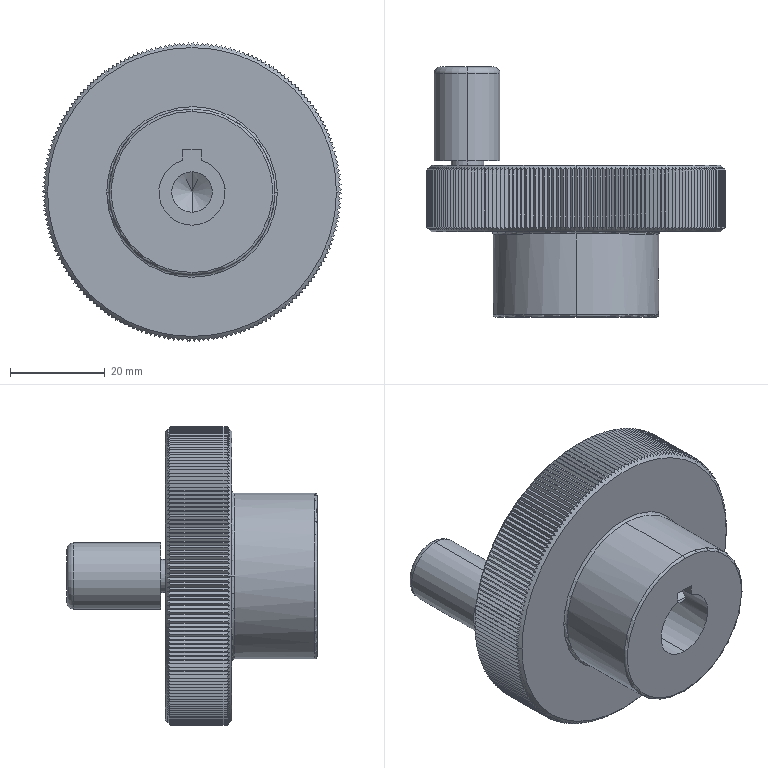Part | STEP file | HBK63_HBK63 | 1 solid | 450 faces | box 62.998 x 52.8 x 62.995 mm | volume 59159 mm3 | plane 418 | cylinder 15 | torus 11 | cone 6 | commonest cylinder face diameters 14 x4 8.933 x3 4.2 x2 7 x2 9.333 x2 35 x2